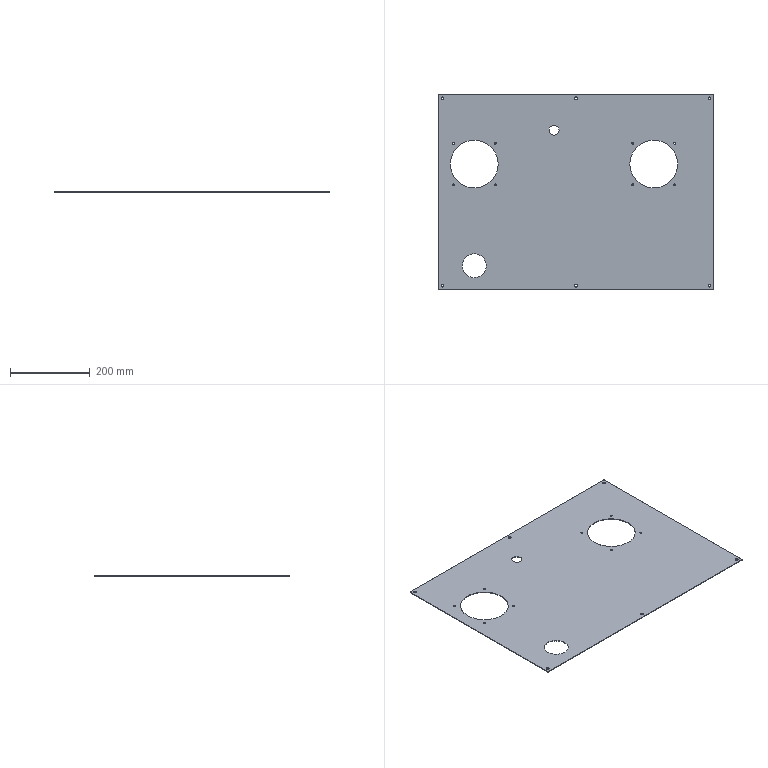Part | NX | 1 solid | 50 faces | box 690 x 490 x 1.5 mm | volume 467655 mm3 | cylinder 40 | plane 6 | cone 4 | commonest cylinder face diameters 5 x16 7 x12 4 x4 120 x4 25 x2 60 x2